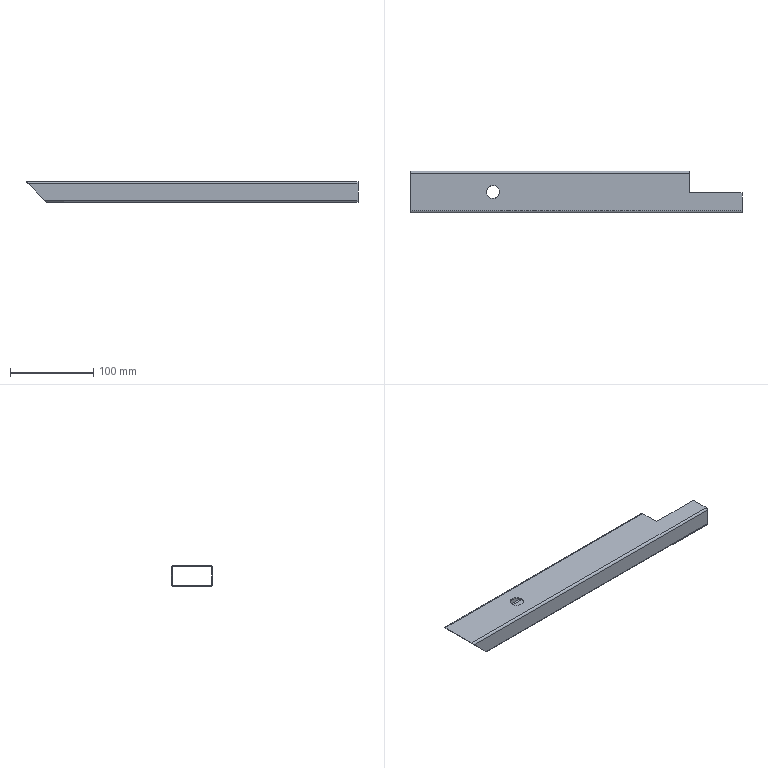Part | STEP file | 5090501L | 1 solid | 25 faces | box 400 x 50 x 25 mm | volume 74106 mm3 | plane 13 | cylinder 12 | commonest cylinder face diameters 2 x4 5 x4 16 x2 3.2 x1 18 x1